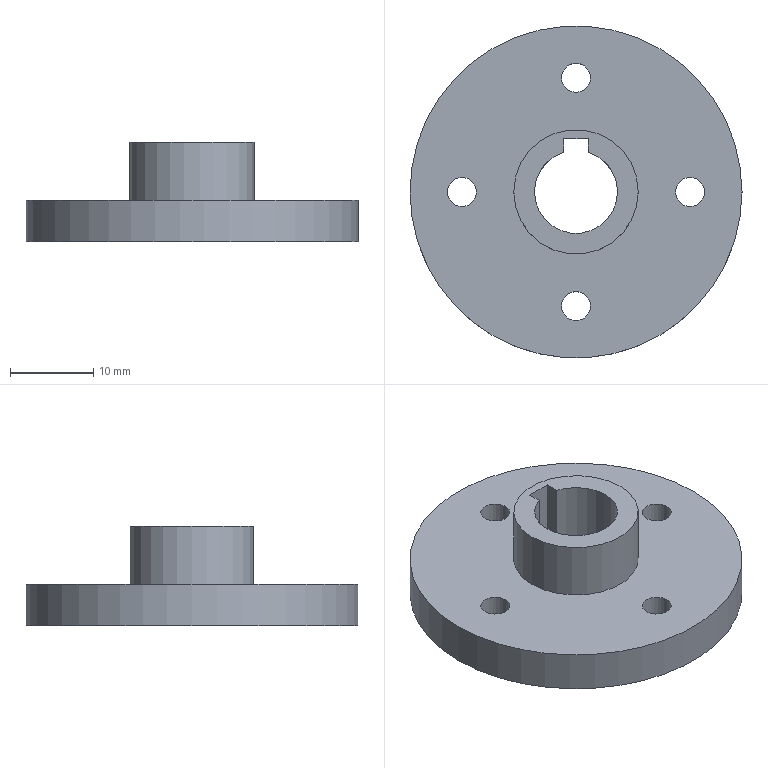Part | NX | features SIMPLE HOLE 5, DATUM_CSYS 4, SYMBOLIC_THREAD 4, SKETCH 3, CPROJ 2, HOLE PACKAGE 2, EXTRUDE 1, SWP104 1 | 1 solid | 15 faces | box 40 x 40 x 12 mm | volume 5639 mm3 | cylinder 8 | plane 7 | commonest cylinder face diameters 3.5 x4 10 x1 15 x1 20 x1 40 x1
STEP:
#1=CARTESIAN_POINT('',(-1.5,4.77,3.));
#2=VERTEX_POINT('',#1);
#3=CARTESIAN_POINT('',(1.5,4.77,3.));
#4=VERTEX_POINT('',#3);
#5=CARTESIAN_POINT('',(0.,0.,3.));
#6=DIRECTION('',(0.,0.,1.));
#7=DIRECTION('',(1.,0.,0.));
#8=AXIS2_PLACEMENT_3D('',#5,#6,#7);
#9=CIRCLE('',#8,5.);
#10=EDGE_CURVE('',#2,#4,#9,.T.);
#11=ORIENTED_EDGE('',*,*,#10,.F.);
#12=CARTESIAN_POINT('',(-1.5,4.77,12.));
#13=VERTEX_POINT('',#12);
#14=CARTESIAN_POINT('',(-1.5,4.77,0.));
#15=DIRECTION('',(0.,0.,-1.));
#16=VECTOR('',#15,1000.);
#17=LINE('',#14,#16);
#18=EDGE_CURVE('',#2,#13,#17,.F.);
#19=ORIENTED_EDGE('',*,*,#18,.T.);
#20=CARTESIAN_POINT('',(1.5,4.77,12.));
#21=VERTEX_POINT('',#20);
#22=CARTESIAN_POINT('',(0.,0.,12.));
#23=DIRECTION('',(0.,0.,-1.));
#24=DIRECTION('',(-1.,0.,0.));
#25=AXIS2_PLACEMENT_3D('',#22,#23,#24);
#26=CIRCLE('',#25,5.);
#27=EDGE_CURVE('',#21,#13,#26,.T.);
#28=ORIENTED_EDGE('',*,*,#27,.F.);
#29=CARTESIAN_POINT('',(1.5,4.77,0.));
#30=DIRECTION('',(0.,0.,-1.));
#31=VECTOR('',#30,1000.);
#32=LINE('',#29,#31);
#33=EDGE_CURVE('',#21,#4,#32,.T.);
#34=ORIENTED_EDGE('',*,*,#33,.T.);
#35=EDGE_LOOP('',(#11,#19,#28,#34));
#36=FACE_BOUND('',#35,.T.);
#37=CARTESIAN_POINT('',(0.,0.,0.));
#38=DIRECTION('',(0.,0.,-1.));
#39=DIRECTION('',(-1.,0.,0.));
#40=AXIS2_PLACEMENT_3D('',#37,#38,#39);
#41=CYLINDRICAL_SURFACE('',#40,5.);
#42=ADVANCED_FACE('',(#36),#41,.F.);
#43=CARTESIAN_POINT('',(-7.5,0.,12.));
#44=VERTEX_POINT('',#43);
#45=CARTESIAN_POINT('',(0.,0.,12.));
#46=DIRECTION('',(0.,0.,-1.));
#47=DIRECTION('',(-1.,0.,0.));
#48=AXIS2_PLACEMENT_3D('',#45,#46,#47);
#49=CIRCLE('',#48,7.5);
#50=EDGE_CURVE('',#44,#44,#49,.T.);
#51=ORIENTED_EDGE('',*,*,#50,.F.);
#52=EDGE_LOOP('',(#51));
#53=FACE_BOUND('',#52,.T.);
#54=ORIENTED_EDGE('',*,*,#27,.T.);
#55=CARTESIAN_POINT('',(-1.5,6.4,12.));
#56=VERTEX_POINT('',#55);
#57=CARTESIAN_POINT('',(-1.5,7.5,12.));
#58=DIRECTION('',(0.,1.,0.));
#59=VECTOR('',#58,1000.);
#60=LINE('',#57,#59);
#61=EDGE_CURVE('',#13,#56,#60,.T.);
#62=ORIENTED_EDGE('',*,*,#61,.T.);
#63=CARTESIAN_POINT('',(1.5,6.4,12.));
#64=VERTEX_POINT('',#63);
#65=CARTESIAN_POINT('',(0.,6.4,12.));
#66=DIRECTION('',(1.,0.,0.));
#67=VECTOR('',#66,1000.);
#68=LINE('',#65,#67);
#69=EDGE_CURVE('',#56,#64,#68,.T.);
#70=ORIENTED_EDGE('',*,*,#69,.T.);
#71=CARTESIAN_POINT('',(1.5,7.5,12.));
#72=DIRECTION('',(0.,-1.,0.));
#73=VECTOR('',#72,1000.);
#74=LINE('',#71,#73);
#75=EDGE_CURVE('',#64,#21,#74,.T.);
#76=ORIENTED_EDGE('',*,*,#75,.T.);
#77=EDGE_LOOP('',(#54,#62,#70,#76));
#78=FACE_BOUND('',#77,.T.);
#79=CARTESIAN_POINT('',(0.,7.5,12.));
#80=DIRECTION('',(0.,0.,1.));
#81=DIRECTION('',(1.,0.,0.));
#82=AXIS2_PLACEMENT_3D('',#79,#80,#81);
#83=PLANE('',#82);
#84=ADVANCED_FACE('',(#53,#78),#83,.T.);
#85=CARTESIAN_POINT('',(10.,0.,3.));
#86=VERTEX_POINT('',#85);
#87=CARTESIAN_POINT('',(0.,0.,3.));
#88=DIRECTION('',(0.,0.,1.));
#89=DIRECTION('',(1.,0.,0.));
#90=AXIS2_PLACEMENT_3D('',#87,#88,#89);
#91=CIRCLE('',#90,10.);
#92=EDGE_CURVE('',#86,#86,#91,.F.);
#93=ORIENTED_EDGE('',*,*,#92,.T.);
#94=EDGE_LOOP('',(#93));
#95=FACE_BOUND('',#94,.T.);
#96=CARTESIAN_POINT('',(-1.5,6.4,3.));
#97=VERTEX_POINT('',#96);
#98=CARTESIAN_POINT('',(-1.5,0.,3.));
#99=DIRECTION('',(0.,1.,0.));
#100=VECTOR('',#99,1000.);
#101=LINE('',#98,#100);
#102=EDGE_CURVE('',#2,#97,#101,.T.);
#103=ORIENTED_EDGE('',*,*,#102,.F.);
#104=ORIENTED_EDGE('',*,*,#10,.T.);
#105=CARTESIAN_POINT('',(1.5,6.4,3.));
#106=VERTEX_POINT('',#105);
#107=CARTESIAN_POINT('',(1.5,0.,3.));
#108=DIRECTION('',(0.,-1.,0.));
#109=VECTOR('',#108,1000.);
#110=LINE('',#107,#109);
#111=EDGE_CURVE('',#106,#4,#110,.T.);
#112=ORIENTED_EDGE('',*,*,#111,.F.);
#113=CARTESIAN_POINT('',(0.,6.4,3.));
#114=DIRECTION('',(1.,0.,0.));
#115=VECTOR('',#114,1000.);
#116=LINE('',#113,#115);
#117=EDGE_CURVE('',#97,#106,#116,.T.);
#118=ORIENTED_EDGE('',*,*,#117,.F.);
#119=EDGE_LOOP('',(#103,#104,#112,#118));
#120=FACE_BOUND('',#119,.T.);
#121=CARTESIAN_POINT('',(0.,0.,3.));
#122=DIRECTION('',(0.,0.,1.));
#123=DIRECTION('',(1.,0.,0.));
#124=AXIS2_PLACEMENT_3D('',#121,#122,#123);
#125=PLANE('',#124);
#126=ADVANCED_FACE('',(#95,#120),#125,.F.);
#127=CARTESIAN_POINT('',(10.,0.,0.));
#128=VERTEX_POINT('',#127);
#129=CARTESIAN_POINT('',(0.,0.,0.));
#130=DIRECTION('',(0.,0.,1.));
#131=DIRECTION('',(1.,0.,0.));
#132=AXIS2_PLACEMENT_3D('',#129,#130,#131);
#133=CIRCLE('',#132,10.);
#134=EDGE_CURVE('',#128,#128,#133,.T.);
#135=ORIENTED_EDGE('',*,*,#134,.T.);
#136=EDGE_LOOP('',(#135));
#137=FACE_BOUND('',#136,.T.);
#138=CARTESIAN_POINT('',(15.5,0.,0.));
#139=VERTEX_POINT('',#138);
#140=CARTESIAN_POINT('',(13.75,0.,0.));
#141=DIRECTION('',(0.,0.,1.));
#142=DIRECTION('',(1.,0.,0.));
#143=AXIS2_PLACEMENT_3D('',#140,#141,#142);
#144=CIRCLE('',#143,1.75);
#145=EDGE_CURVE('',#139,#139,#144,.T.);
#146=ORIENTED_EDGE('',*,*,#145,.T.);
#147=EDGE_LOOP('',(#146));
#148=FACE_BOUND('',#147,.T.);
#149=CARTESIAN_POINT('',(1.75,13.75,0.));
#150=VERTEX_POINT('',#149);
#151=CARTESIAN_POINT('',(0.,13.75,0.));
#152=DIRECTION('',(0.,0.,1.));
#153=DIRECTION('',(1.,0.,0.));
#154=AXIS2_PLACEMENT_3D('',#151,#152,#153);
#155=CIRCLE('',#154,1.75);
#156=EDGE_CURVE('',#150,#150,#155,.T.);
#157=ORIENTED_EDGE('',*,*,#156,.T.);
#158=EDGE_LOOP('',(#157));
#159=FACE_BOUND('',#158,.T.);
#160=CARTESIAN_POINT('',(1.75,-13.75,0.));
#161=VERTEX_POINT('',#160);
#162=CARTESIAN_POINT('',(0.,-13.75,0.));
#163=DIRECTION('',(0.,0.,1.));
#164=DIRECTION('',(1.,0.,0.));
#165=AXIS2_PLACEMENT_3D('',#162,#163,#164);
#166=CIRCLE('',#165,1.75);
#167=EDGE_CURVE('',#161,#161,#166,.T.);
#168=ORIENTED_EDGE('',*,*,#167,.T.);
#169=EDGE_LOOP('',(#168));
#170=FACE_BOUND('',#169,.T.);
#171=CARTESIAN_POINT('',(-12.,0.,0.));
#172=VERTEX_POINT('',#171);
#173=CARTESIAN_POINT('',(-13.75,0.,0.));
#174=DIRECTION('',(0.,0.,1.));
#175=DIRECTION('',(1.,0.,0.));
#176=AXIS2_PLACEMENT_3D('',#173,#174,#175);
#177=CIRCLE('',#176,1.75);
#178=EDGE_CURVE('',#172,#172,#177,.T.);
#179=ORIENTED_EDGE('',*,*,#178,.T.);
#180=EDGE_LOOP('',(#179));
#181=FACE_BOUND('',#180,.T.);
#182=CARTESIAN_POINT('',(-20.,0.,0.));
#183=VERTEX_POINT('',#182);
#184=CARTESIAN_POINT('',(0.,0.,0.));
#185=DIRECTION('',(0.,0.,-1.));
#186=DIRECTION('',(-1.,0.,0.));
#187=AXIS2_PLACEMENT_3D('',#184,#185,#186);
#188=CIRCLE('',#187,20.);
#189=EDGE_CURVE('',#183,#183,#188,.T.);
#190=ORIENTED_EDGE('',*,*,#189,.T.);
#191=EDGE_LOOP('',(#190));
#192=FACE_BOUND('',#191,.T.);
#193=CARTESIAN_POINT('',(0.,5.,0.));
#194=DIRECTION('',(0.,0.,-1.));
#195=DIRECTION('',(-1.,0.,0.));
#196=AXIS2_PLACEMENT_3D('',#193,#194,#195);
#197=PLANE('',#196);
#198=ADVANCED_FACE('',(#137,#148,#159,#170,#181,#192),#197,.T.);
#199=CARTESIAN_POINT('',(-20.,0.,5.));
#200=VERTEX_POINT('',#199);
#201=CARTESIAN_POINT('',(0.,0.,5.));
#202=DIRECTION('',(0.,0.,-1.));
#203=DIRECTION('',(-1.,0.,0.));
#204=AXIS2_PLACEMENT_3D('',#201,#202,#203);
#205=CIRCLE('',#204,20.);
#206=EDGE_CURVE('',#200,#200,#205,.T.);
#207=ORIENTED_EDGE('',*,*,#206,.T.);
#208=EDGE_LOOP('',(#207));
#209=FACE_BOUND('',#208,.T.);
#210=ORIENTED_EDGE('',*,*,#189,.F.);
#211=EDGE_LOOP('',(#210));
#212=FACE_BOUND('',#211,.T.);
#213=CARTESIAN_POINT('',(0.,0.,0.));
#214=DIRECTION('',(0.,0.,-1.));
#215=DIRECTION('',(-1.,0.,0.));
#216=AXIS2_PLACEMENT_3D('',#213,#214,#215);
#217=CYLINDRICAL_SURFACE('',#216,20.);
#218=ADVANCED_FACE('',(#209,#212),#217,.T.);
#219=CARTESIAN_POINT('',(15.5,0.,5.));
#220=VERTEX_POINT('',#219);
#221=CARTESIAN_POINT('',(13.75,0.,5.));
#222=DIRECTION('',(0.,0.,1.));
#223=DIRECTION('',(1.,0.,0.));
#224=AXIS2_PLACEMENT_3D('',#221,#222,#223);
#225=CIRCLE('',#224,1.75);
#226=EDGE_CURVE('',#220,#220,#225,.T.);
#227=ORIENTED_EDGE('',*,*,#226,.F.);
#228=EDGE_LOOP('',(#227));
#229=FACE_BOUND('',#228,.T.);
#230=CARTESIAN_POINT('',(1.75,13.75,5.));
#231=VERTEX_POINT('',#230);
#232=CARTESIAN_POINT('',(0.,13.75,5.));
#233=DIRECTION('',(0.,0.,1.));
#234=DIRECTION('',(1.,0.,0.));
#235=AXIS2_PLACEMENT_3D('',#232,#233,#234);
#236=CIRCLE('',#235,1.75);
#237=EDGE_CURVE('',#231,#231,#236,.T.);
#238=ORIENTED_EDGE('',*,*,#237,.F.);
#239=EDGE_LOOP('',(#238));
#240=FACE_BOUND('',#239,.T.);
#241=CARTESIAN_POINT('',(1.75,-13.75,5.));
#242=VERTEX_POINT('',#241);
#243=CARTESIAN_POINT('',(0.,-13.75,5.));
#244=DIRECTION('',(0.,0.,1.));
#245=DIRECTION('',(1.,0.,0.));
#246=AXIS2_PLACEMENT_3D('',#243,#244,#245);
#247=CIRCLE('',#246,1.75);
#248=EDGE_CURVE('',#242,#242,#247,.T.);
#249=ORIENTED_EDGE('',*,*,#248,.F.);
#250=EDGE_LOOP('',(#249));
#251=FACE_BOUND('',#250,.T.);
#252=CARTESIAN_POINT('',(-12.,0.,5.));
#253=VERTEX_POINT('',#252);
#254=CARTESIAN_POINT('',(-13.75,0.,5.));
#255=DIRECTION('',(0.,0.,1.));
#256=DIRECTION('',(1.,0.,0.));
#257=AXIS2_PLACEMENT_3D('',#254,#255,#256);
#258=CIRCLE('',#257,1.75);
#259=EDGE_CURVE('',#253,#253,#258,.T.);
#260=ORIENTED_EDGE('',*,*,#259,.F.);
#261=EDGE_LOOP('',(#260));
#262=FACE_BOUND('',#261,.T.);
#263=CARTESIAN_POINT('',(-7.5,0.,5.));
#264=VERTEX_POINT('',#263);
#265=CARTESIAN_POINT('',(0.,0.,5.));
#266=DIRECTION('',(0.,0.,-1.));
#267=DIRECTION('',(-1.,0.,0.));
#268=AXIS2_PLACEMENT_3D('',#265,#266,#267);
#269=CIRCLE('',#268,7.5);
#270=EDGE_CURVE('',#264,#264,#269,.T.);
#271=ORIENTED_EDGE('',*,*,#270,.T.);
#272=EDGE_LOOP('',(#271));
#273=FACE_BOUND('',#272,.T.);
#274=ORIENTED_EDGE('',*,*,#206,.F.);
#275=EDGE_LOOP('',(#274));
#276=FACE_BOUND('',#275,.T.);
#277=CARTESIAN_POINT('',(0.,20.,5.));
#278=DIRECTION('',(0.,0.,1.));
#279=DIRECTION('',(1.,0.,0.));
#280=AXIS2_PLACEMENT_3D('',#277,#278,#279);
#281=PLANE('',#280);
#282=ADVANCED_FACE('',(#229,#240,#251,#262,#273,#276),#281,.T.);
#283=ORIENTED_EDGE('',*,*,#50,.T.);
#284=EDGE_LOOP('',(#283));
#285=FACE_BOUND('',#284,.T.);
#286=ORIENTED_EDGE('',*,*,#270,.F.);
#287=EDGE_LOOP('',(#286));
#288=FACE_BOUND('',#287,.T.);
#289=CARTESIAN_POINT('',(0.,0.,0.));
#290=DIRECTION('',(0.,0.,-1.));
#291=DIRECTION('',(-1.,0.,0.));
#292=AXIS2_PLACEMENT_3D('',#289,#290,#291);
#293=CYLINDRICAL_SURFACE('',#292,7.5);
#294=ADVANCED_FACE('',(#285,#288),#293,.T.);
#295=ORIENTED_EDGE('',*,*,#259,.T.);
#296=EDGE_LOOP('',(#295));
#297=FACE_BOUND('',#296,.T.);
#298=ORIENTED_EDGE('',*,*,#178,.F.);
#299=EDGE_LOOP('',(#298));
#300=FACE_BOUND('',#299,.T.);
#301=CARTESIAN_POINT('',(-13.75,0.,0.));
#302=DIRECTION('',(0.,0.,1.));
#303=DIRECTION('',(1.,0.,0.));
#304=AXIS2_PLACEMENT_3D('',#301,#302,#303);
#305=CYLINDRICAL_SURFACE('',#304,1.75);
#306=ADVANCED_FACE('',(#297,#300),#305,.F.);
#307=ORIENTED_EDGE('',*,*,#248,.T.);
#308=EDGE_LOOP('',(#307));
#309=FACE_BOUND('',#308,.T.);
#310=ORIENTED_EDGE('',*,*,#167,.F.);
#311=EDGE_LOOP('',(#310));
#312=FACE_BOUND('',#311,.T.);
#313=CARTESIAN_POINT('',(0.,-13.75,0.));
#314=DIRECTION('',(0.,0.,1.));
#315=DIRECTION('',(1.,0.,0.));
#316=AXIS2_PLACEMENT_3D('',#313,#314,#315);
#317=CYLINDRICAL_SURFACE('',#316,1.75);
#318=ADVANCED_FACE('',(#309,#312),#317,.F.);
#319=ORIENTED_EDGE('',*,*,#237,.T.);
#320=EDGE_LOOP('',(#319));
#321=FACE_BOUND('',#320,.T.);
#322=ORIENTED_EDGE('',*,*,#156,.F.);
#323=EDGE_LOOP('',(#322));
#324=FACE_BOUND('',#323,.T.);
#325=CARTESIAN_POINT('',(0.,13.75,0.));
#326=DIRECTION('',(0.,0.,1.));
#327=DIRECTION('',(1.,0.,0.));
#328=AXIS2_PLACEMENT_3D('',#325,#326,#327);
#329=CYLINDRICAL_SURFACE('',#328,1.75);
#330=ADVANCED_FACE('',(#321,#324),#329,.F.);
#331=ORIENTED_EDGE('',*,*,#226,.T.);
#332=EDGE_LOOP('',(#331));
#333=FACE_BOUND('',#332,.T.);
#334=ORIENTED_EDGE('',*,*,#145,.F.);
#335=EDGE_LOOP('',(#334));
#336=FACE_BOUND('',#335,.T.);
#337=CARTESIAN_POINT('',(13.75,0.,0.));
#338=DIRECTION('',(0.,0.,1.));
#339=DIRECTION('',(1.,0.,0.));
#340=AXIS2_PLACEMENT_3D('',#337,#338,#339);
#341=CYLINDRICAL_SURFACE('',#340,1.75);
#342=ADVANCED_FACE('',(#333,#336),#341,.F.);
#343=ORIENTED_EDGE('',*,*,#92,.F.);
#344=EDGE_LOOP('',(#343));
#345=FACE_BOUND('',#344,.T.);
#346=ORIENTED_EDGE('',*,*,#134,.F.);
#347=EDGE_LOOP('',(#346));
#348=FACE_BOUND('',#347,.T.);
#349=CARTESIAN_POINT('',(0.,0.,0.));
#350=DIRECTION('',(0.,0.,1.));
#351=DIRECTION('',(1.,0.,0.));
#352=AXIS2_PLACEMENT_3D('',#349,#350,#351);
#353=CYLINDRICAL_SURFACE('',#352,10.);
#354=ADVANCED_FACE('',(#345,#348),#353,.F.);
#355=CARTESIAN_POINT('',(-1.5,6.4,50.));
#356=DIRECTION('',(0.,0.,-1.));
#357=VECTOR('',#356,1000.);
#358=LINE('',#355,#357);
#359=EDGE_CURVE('',#97,#56,#358,.F.);
#360=ORIENTED_EDGE('',*,*,#359,.F.);
#361=ORIENTED_EDGE('',*,*,#117,.T.);
#362=CARTESIAN_POINT('',(1.5,6.4,50.));
#363=DIRECTION('',(0.,0.,-1.));
#364=VECTOR('',#363,1000.);
#365=LINE('',#362,#364);
#366=EDGE_CURVE('',#106,#64,#365,.F.);
#367=ORIENTED_EDGE('',*,*,#366,.T.);
#368=ORIENTED_EDGE('',*,*,#69,.F.);
#369=EDGE_LOOP('',(#360,#361,#367,#368));
#370=FACE_BOUND('',#369,.T.);
#371=CARTESIAN_POINT('',(1.5,6.4,50.));
#372=DIRECTION('',(0.,-1.,0.));
#373=DIRECTION('',(0.,0.,-1.));
#374=AXIS2_PLACEMENT_3D('',#371,#372,#373);
#375=PLANE('',#374);
#376=ADVANCED_FACE('',(#370),#375,.T.);
#377=ORIENTED_EDGE('',*,*,#18,.F.);
#378=ORIENTED_EDGE('',*,*,#102,.T.);
#379=ORIENTED_EDGE('',*,*,#359,.T.);
#380=ORIENTED_EDGE('',*,*,#61,.F.);
#381=EDGE_LOOP('',(#377,#378,#379,#380));
#382=FACE_BOUND('',#381,.T.);
#383=CARTESIAN_POINT('',(-1.5,6.4,50.));
#384=DIRECTION('',(1.,0.,0.));
#385=DIRECTION('',(0.,1.,0.));
#386=AXIS2_PLACEMENT_3D('',#383,#384,#385);
#387=PLANE('',#386);
#388=ADVANCED_FACE('',(#382),#387,.T.);
#389=ORIENTED_EDGE('',*,*,#366,.F.);
#390=ORIENTED_EDGE('',*,*,#111,.T.);
#391=ORIENTED_EDGE('',*,*,#33,.F.);
#392=ORIENTED_EDGE('',*,*,#75,.F.);
#393=EDGE_LOOP('',(#389,#390,#391,#392));
#394=FACE_BOUND('',#393,.T.);
#395=CARTESIAN_POINT('',(1.5,0.,50.));
#396=DIRECTION('',(-1.,0.,0.));
#397=DIRECTION('',(0.,0.,1.));
#398=AXIS2_PLACEMENT_3D('',#395,#396,#397);
#399=PLANE('',#398);
#400=ADVANCED_FACE('',(#394),#399,.T.);
#401=CLOSED_SHELL('',(#42,#84,#126,#198,#218,#282,#294,#306,#318,#330,#342,#354,#376,#388,#400));
#402=MANIFOLD_SOLID_BREP('',#401);
#403=(LENGTH_UNIT()NAMED_UNIT(*)SI_UNIT(.MILLI.,.METRE.));
#404=UNCERTAINTY_MEASURE_WITH_UNIT(LENGTH_MEASURE(0.00001),#403,'','');
#405=(NAMED_UNIT(*)PLANE_ANGLE_UNIT()SI_UNIT($,.RADIAN.));
#406=(NAMED_UNIT(*)SI_UNIT($,.STERADIAN.)SOLID_ANGLE_UNIT());
#407=(GEOMETRIC_REPRESENTATION_CONTEXT(3)GLOBAL_UNCERTAINTY_ASSIGNED_CONTEXT((#404))GLOBAL_UNIT_ASSIGNED_CONTEXT((#403,#405,#406))REPRESENTATION_CONTEXT('',''));
#408=ADVANCED_BREP_SHAPE_REPRESENTATION('',(#402),#407);